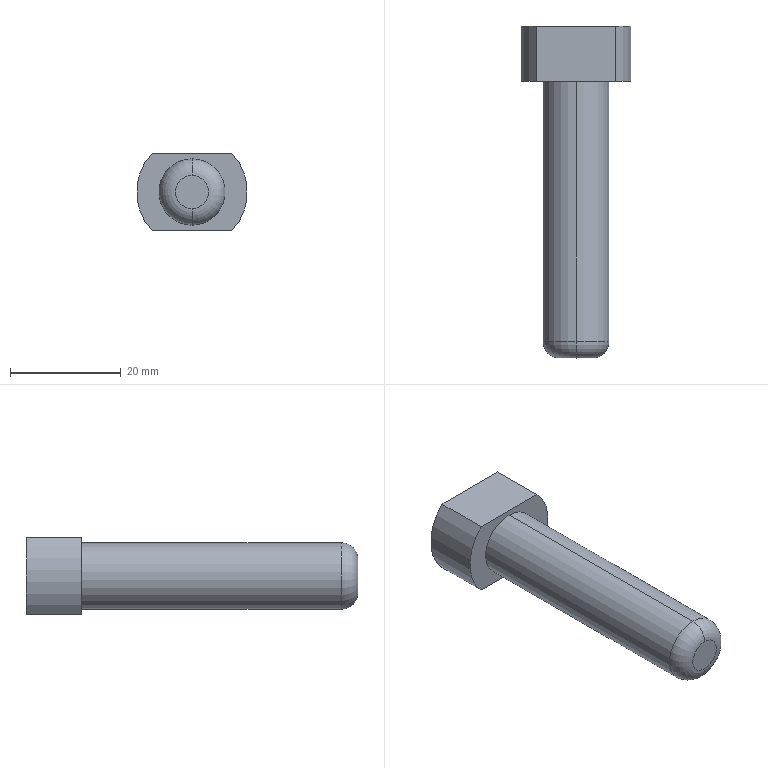Part | SolidWorks | features ICE 2, Extrusion 1, Fillet 1 | 1 solid | 11 faces | box 20 x 60 x 14 mm | volume 8141 mm3 | plane 5 | cylinder 4 | torus 2 | commonest cylinder face diameters 12 x2 20 x2
STEP:
#1=CARTESIAN_POINT('',(0.,-30.,-3.));
#2=VERTEX_POINT('',#1);
#3=CARTESIAN_POINT('',(0.,-30.,3.));
#4=VERTEX_POINT('',#3);
#5=CARTESIAN_POINT('',(0.,-30.,0.));
#6=DIRECTION('',(0.,-1.,0.));
#7=DIRECTION('',(0.,0.,1.));
#8=AXIS2_PLACEMENT_3D('',#5,#6,#7);
#9=CIRCLE('',#8,3.);
#10=EDGE_CURVE('',#2,#4,#9,.T.);
#11=ORIENTED_EDGE('',*,*,#10,.F.);
#12=CARTESIAN_POINT('',(0.,-27.,-6.));
#13=VERTEX_POINT('',#12);
#14=CARTESIAN_POINT('',(0.,-27.,-3.));
#15=DIRECTION('',(1.,0.,0.));
#16=DIRECTION('',(0.,0.,-1.));
#17=AXIS2_PLACEMENT_3D('',#14,#15,#16);
#18=CIRCLE('',#17,3.);
#19=EDGE_CURVE('',#2,#13,#18,.T.);
#20=ORIENTED_EDGE('',*,*,#19,.T.);
#21=CARTESIAN_POINT('',(0.,-27.,6.));
#22=VERTEX_POINT('',#21);
#23=CARTESIAN_POINT('',(0.,-27.,0.));
#24=DIRECTION('',(0.,1.,0.));
#25=DIRECTION('',(0.,0.,1.));
#26=AXIS2_PLACEMENT_3D('',#23,#24,#25);
#27=CIRCLE('',#26,6.);
#28=EDGE_CURVE('',#22,#13,#27,.T.);
#29=ORIENTED_EDGE('',*,*,#28,.F.);
#30=CARTESIAN_POINT('',(0.,-27.,3.));
#31=DIRECTION('',(-1.,0.,0.));
#32=DIRECTION('',(0.,0.,1.));
#33=AXIS2_PLACEMENT_3D('',#30,#31,#32);
#34=CIRCLE('',#33,3.);
#35=EDGE_CURVE('',#4,#22,#34,.T.);
#36=ORIENTED_EDGE('',*,*,#35,.F.);
#37=EDGE_LOOP('',(#11,#20,#29,#36));
#38=FACE_OUTER_BOUND('',#37,.T.);
#39=CARTESIAN_POINT('',(0.,-27.,0.));
#40=DIRECTION('',(0.,1.,0.));
#41=DIRECTION('',(0.,0.,1.));
#42=AXIS2_PLACEMENT_3D('',#39,#40,#41);
#43=TOROIDAL_SURFACE('',#42,3.,3.);
#44=ADVANCED_FACE('',(#38),#43,.T.);
#45=CARTESIAN_POINT('',(0.,20.,-6.));
#46=VERTEX_POINT('',#45);
#47=CARTESIAN_POINT('',(0.,20.,6.));
#48=VERTEX_POINT('',#47);
#49=CARTESIAN_POINT('',(0.,20.,0.));
#50=DIRECTION('',(0.,-1.,0.));
#51=DIRECTION('',(0.,0.,-1.));
#52=AXIS2_PLACEMENT_3D('',#49,#50,#51);
#53=CIRCLE('',#52,6.);
#54=EDGE_CURVE('',#46,#48,#53,.T.);
#55=ORIENTED_EDGE('',*,*,#54,.T.);
#56=CARTESIAN_POINT('',(0.,20.,6.));
#57=DIRECTION('',(0.,-1.,0.));
#58=VECTOR('',#57,1000.);
#59=LINE('',#56,#58);
#60=EDGE_CURVE('',#48,#22,#59,.T.);
#61=ORIENTED_EDGE('',*,*,#60,.T.);
#62=ORIENTED_EDGE('',*,*,#28,.T.);
#63=CARTESIAN_POINT('',(0.,20.,-6.));
#64=DIRECTION('',(0.,-1.,0.));
#65=VECTOR('',#64,1000.);
#66=LINE('',#63,#65);
#67=EDGE_CURVE('',#46,#13,#66,.T.);
#68=ORIENTED_EDGE('',*,*,#67,.F.);
#69=EDGE_LOOP('',(#55,#61,#62,#68));
#70=FACE_OUTER_BOUND('',#69,.T.);
#71=CARTESIAN_POINT('',(0.,20.,0.));
#72=DIRECTION('',(0.,-1.,0.));
#73=DIRECTION('',(0.,0.,-1.));
#74=AXIS2_PLACEMENT_3D('',#71,#72,#73);
#75=CYLINDRICAL_SURFACE('',#74,6.);
#76=ADVANCED_FACE('',(#70),#75,.T.);
#77=CARTESIAN_POINT('',(-7.141,30.,-7.));
#78=VERTEX_POINT('',#77);
#79=CARTESIAN_POINT('',(-7.141,30.,7.));
#80=VERTEX_POINT('',#79);
#81=CARTESIAN_POINT('',(0.,30.,0.));
#82=DIRECTION('',(0.,1.,0.));
#83=DIRECTION('',(0.,0.,1.));
#84=AXIS2_PLACEMENT_3D('',#81,#82,#83);
#85=CIRCLE('',#84,10.);
#86=EDGE_CURVE('',#78,#80,#85,.T.);
#87=ORIENTED_EDGE('',*,*,#86,.F.);
#88=CARTESIAN_POINT('',(-7.141,20.,-7.));
#89=VERTEX_POINT('',#88);
#90=CARTESIAN_POINT('',(-7.141,20.,-7.));
#91=DIRECTION('',(0.,1.,0.));
#92=VECTOR('',#91,1000.);
#93=LINE('',#90,#92);
#94=EDGE_CURVE('',#89,#78,#93,.T.);
#95=ORIENTED_EDGE('',*,*,#94,.F.);
#96=CARTESIAN_POINT('',(-7.141,20.,7.));
#97=VERTEX_POINT('',#96);
#98=CARTESIAN_POINT('',(0.,20.,0.));
#99=DIRECTION('',(0.,-1.,0.));
#100=DIRECTION('',(0.,0.,-1.));
#101=AXIS2_PLACEMENT_3D('',#98,#99,#100);
#102=CIRCLE('',#101,10.);
#103=EDGE_CURVE('',#97,#89,#102,.T.);
#104=ORIENTED_EDGE('',*,*,#103,.F.);
#105=CARTESIAN_POINT('',(-7.141,20.,7.));
#106=DIRECTION('',(0.,1.,0.));
#107=VECTOR('',#106,1000.);
#108=LINE('',#105,#107);
#109=EDGE_CURVE('',#97,#80,#108,.T.);
#110=ORIENTED_EDGE('',*,*,#109,.T.);
#111=EDGE_LOOP('',(#87,#95,#104,#110));
#112=FACE_OUTER_BOUND('',#111,.T.);
#113=CARTESIAN_POINT('',(0.,30.,0.));
#114=DIRECTION('',(0.,-1.,0.));
#115=DIRECTION('',(0.,0.,-1.));
#116=AXIS2_PLACEMENT_3D('',#113,#114,#115);
#117=CYLINDRICAL_SURFACE('',#116,10.);
#118=ADVANCED_FACE('',(#112),#117,.T.);
#119=CARTESIAN_POINT('',(7.141,20.,-7.));
#120=VERTEX_POINT('',#119);
#121=CARTESIAN_POINT('',(7.141,20.,7.));
#122=VERTEX_POINT('',#121);
#123=CARTESIAN_POINT('',(0.,20.,0.));
#124=DIRECTION('',(0.,-1.,0.));
#125=DIRECTION('',(0.,0.,-1.));
#126=AXIS2_PLACEMENT_3D('',#123,#124,#125);
#127=CIRCLE('',#126,10.);
#128=EDGE_CURVE('',#120,#122,#127,.T.);
#129=ORIENTED_EDGE('',*,*,#128,.F.);
#130=CARTESIAN_POINT('',(7.141,30.,-7.));
#131=VERTEX_POINT('',#130);
#132=CARTESIAN_POINT('',(7.141,20.,-7.));
#133=DIRECTION('',(0.,1.,0.));
#134=VECTOR('',#133,1000.);
#135=LINE('',#132,#134);
#136=EDGE_CURVE('',#120,#131,#135,.T.);
#137=ORIENTED_EDGE('',*,*,#136,.T.);
#138=CARTESIAN_POINT('',(7.141,30.,7.));
#139=VERTEX_POINT('',#138);
#140=CARTESIAN_POINT('',(0.,30.,0.));
#141=DIRECTION('',(0.,1.,0.));
#142=DIRECTION('',(0.,0.,1.));
#143=AXIS2_PLACEMENT_3D('',#140,#141,#142);
#144=CIRCLE('',#143,10.);
#145=EDGE_CURVE('',#139,#131,#144,.T.);
#146=ORIENTED_EDGE('',*,*,#145,.F.);
#147=CARTESIAN_POINT('',(7.141,20.,7.));
#148=DIRECTION('',(0.,1.,0.));
#149=VECTOR('',#148,1000.);
#150=LINE('',#147,#149);
#151=EDGE_CURVE('',#122,#139,#150,.T.);
#152=ORIENTED_EDGE('',*,*,#151,.F.);
#153=EDGE_LOOP('',(#129,#137,#146,#152));
#154=FACE_OUTER_BOUND('',#153,.T.);
#155=CARTESIAN_POINT('',(0.,30.,0.));
#156=DIRECTION('',(0.,-1.,0.));
#157=DIRECTION('',(0.,0.,-1.));
#158=AXIS2_PLACEMENT_3D('',#155,#156,#157);
#159=CYLINDRICAL_SURFACE('',#158,10.);
#160=ADVANCED_FACE('',(#154),#159,.T.);
#161=CARTESIAN_POINT('',(-7.141,30.,-7.));
#162=DIRECTION('',(1.,0.,0.));
#163=VECTOR('',#162,1000.);
#164=LINE('',#161,#163);
#165=EDGE_CURVE('',#78,#131,#164,.T.);
#166=ORIENTED_EDGE('',*,*,#165,.F.);
#167=ORIENTED_EDGE('',*,*,#86,.T.);
#168=CARTESIAN_POINT('',(-7.141,30.,7.));
#169=DIRECTION('',(-1.,0.,0.));
#170=VECTOR('',#169,1000.);
#171=LINE('',#168,#170);
#172=EDGE_CURVE('',#139,#80,#171,.T.);
#173=ORIENTED_EDGE('',*,*,#172,.F.);
#174=ORIENTED_EDGE('',*,*,#145,.T.);
#175=EDGE_LOOP('',(#166,#167,#173,#174));
#176=FACE_OUTER_BOUND('',#175,.T.);
#177=CARTESIAN_POINT('',(0.,30.,0.));
#178=DIRECTION('',(0.,1.,0.));
#179=DIRECTION('',(0.,0.,1.));
#180=AXIS2_PLACEMENT_3D('',#177,#178,#179);
#181=PLANE('',#180);
#182=ADVANCED_FACE('',(#176),#181,.T.);
#183=CARTESIAN_POINT('',(-7.141,20.,-7.));
#184=DIRECTION('',(1.,0.,0.));
#185=VECTOR('',#184,1000.);
#186=LINE('',#183,#185);
#187=EDGE_CURVE('',#89,#120,#186,.T.);
#188=ORIENTED_EDGE('',*,*,#187,.T.);
#189=ORIENTED_EDGE('',*,*,#128,.T.);
#190=CARTESIAN_POINT('',(-7.141,20.,7.));
#191=DIRECTION('',(-1.,0.,0.));
#192=VECTOR('',#191,1000.);
#193=LINE('',#190,#192);
#194=EDGE_CURVE('',#122,#97,#193,.T.);
#195=ORIENTED_EDGE('',*,*,#194,.T.);
#196=ORIENTED_EDGE('',*,*,#103,.T.);
#197=EDGE_LOOP('',(#188,#189,#195,#196));
#198=FACE_OUTER_BOUND('',#197,.T.);
#199=ORIENTED_EDGE('',*,*,#54,.F.);
#200=CARTESIAN_POINT('',(0.,20.,0.));
#201=DIRECTION('',(0.,-1.,0.));
#202=DIRECTION('',(0.,0.,-1.));
#203=AXIS2_PLACEMENT_3D('',#200,#201,#202);
#204=CIRCLE('',#203,6.);
#205=EDGE_CURVE('',#48,#46,#204,.T.);
#206=ORIENTED_EDGE('',*,*,#205,.F.);
#207=EDGE_LOOP('',(#199,#206));
#208=FACE_BOUND('',#207,.T.);
#209=CARTESIAN_POINT('',(0.,20.,0.));
#210=DIRECTION('',(0.,-1.,0.));
#211=DIRECTION('',(0.,0.,-1.));
#212=AXIS2_PLACEMENT_3D('',#209,#210,#211);
#213=PLANE('',#212);
#214=ADVANCED_FACE('',(#198,#208),#213,.T.);
#215=ORIENTED_EDGE('',*,*,#60,.F.);
#216=ORIENTED_EDGE('',*,*,#205,.T.);
#217=ORIENTED_EDGE('',*,*,#67,.T.);
#218=CARTESIAN_POINT('',(0.,-27.,0.));
#219=DIRECTION('',(0.,1.,0.));
#220=DIRECTION('',(0.,0.,1.));
#221=AXIS2_PLACEMENT_3D('',#218,#219,#220);
#222=CIRCLE('',#221,6.);
#223=EDGE_CURVE('',#13,#22,#222,.T.);
#224=ORIENTED_EDGE('',*,*,#223,.T.);
#225=EDGE_LOOP('',(#215,#216,#217,#224));
#226=FACE_OUTER_BOUND('',#225,.T.);
#227=CARTESIAN_POINT('',(0.,20.,0.));
#228=DIRECTION('',(0.,-1.,0.));
#229=DIRECTION('',(0.,0.,-1.));
#230=AXIS2_PLACEMENT_3D('',#227,#228,#229);
#231=CYLINDRICAL_SURFACE('',#230,6.);
#232=ADVANCED_FACE('',(#226),#231,.T.);
#233=CARTESIAN_POINT('',(0.,-30.,0.));
#234=DIRECTION('',(0.,-1.,0.));
#235=DIRECTION('',(0.,0.,1.));
#236=AXIS2_PLACEMENT_3D('',#233,#234,#235);
#237=CIRCLE('',#236,3.);
#238=EDGE_CURVE('',#4,#2,#237,.T.);
#239=ORIENTED_EDGE('',*,*,#238,.T.);
#240=ORIENTED_EDGE('',*,*,#10,.T.);
#241=EDGE_LOOP('',(#239,#240));
#242=FACE_OUTER_BOUND('',#241,.T.);
#243=CARTESIAN_POINT('',(0.,-30.,0.));
#244=DIRECTION('',(0.,1.,0.));
#245=DIRECTION('',(0.,0.,1.));
#246=AXIS2_PLACEMENT_3D('',#243,#244,#245);
#247=PLANE('',#246);
#248=ADVANCED_FACE('',(#242),#247,.F.);
#249=ORIENTED_EDGE('',*,*,#19,.F.);
#250=ORIENTED_EDGE('',*,*,#238,.F.);
#251=ORIENTED_EDGE('',*,*,#35,.T.);
#252=ORIENTED_EDGE('',*,*,#223,.F.);
#253=EDGE_LOOP('',(#249,#250,#251,#252));
#254=FACE_OUTER_BOUND('',#253,.T.);
#255=CARTESIAN_POINT('',(0.,-27.,0.));
#256=DIRECTION('',(0.,1.,0.));
#257=DIRECTION('',(0.,0.,1.));
#258=AXIS2_PLACEMENT_3D('',#255,#256,#257);
#259=TOROIDAL_SURFACE('',#258,3.,3.);
#260=ADVANCED_FACE('',(#254),#259,.T.);
#261=ORIENTED_EDGE('',*,*,#172,.T.);
#262=ORIENTED_EDGE('',*,*,#109,.F.);
#263=ORIENTED_EDGE('',*,*,#194,.F.);
#264=ORIENTED_EDGE('',*,*,#151,.T.);
#265=EDGE_LOOP('',(#261,#262,#263,#264));
#266=FACE_OUTER_BOUND('',#265,.T.);
#267=CARTESIAN_POINT('',(-7.141,20.,7.));
#268=DIRECTION('',(0.,0.,-1.));
#269=DIRECTION('',(-1.,0.,0.));
#270=AXIS2_PLACEMENT_3D('',#267,#268,#269);
#271=PLANE('',#270);
#272=ADVANCED_FACE('',(#266),#271,.F.);
#273=ORIENTED_EDGE('',*,*,#165,.T.);
#274=ORIENTED_EDGE('',*,*,#136,.F.);
#275=ORIENTED_EDGE('',*,*,#187,.F.);
#276=ORIENTED_EDGE('',*,*,#94,.T.);
#277=EDGE_LOOP('',(#273,#274,#275,#276));
#278=FACE_OUTER_BOUND('',#277,.T.);
#279=CARTESIAN_POINT('',(-7.141,20.,-7.));
#280=DIRECTION('',(0.,0.,1.));
#281=DIRECTION('',(1.,0.,0.));
#282=AXIS2_PLACEMENT_3D('',#279,#280,#281);
#283=PLANE('',#282);
#284=ADVANCED_FACE('',(#278),#283,.F.);
#285=CLOSED_SHELL('',(#44,#76,#118,#160,#182,#214,#232,#248,#260,#272,#284));
#286=MANIFOLD_SOLID_BREP('',#285);
#287=CARTESIAN_POINT('',(0.,0.,0.));
#288=DIRECTION('',(0.,0.,1.));
#289=DIRECTION('',(1.,0.,0.));
#290=AXIS2_PLACEMENT_3D('',#287,#288,#289);
#291=(LENGTH_UNIT()NAMED_UNIT(*)SI_UNIT(.MILLI.,.METRE.));
#292=UNCERTAINTY_MEASURE_WITH_UNIT(LENGTH_MEASURE(0.00001),#291,'','');
#293=(NAMED_UNIT(*)PLANE_ANGLE_UNIT()SI_UNIT($,.RADIAN.));
#294=(NAMED_UNIT(*)SI_UNIT($,.STERADIAN.)SOLID_ANGLE_UNIT());
#295=(GEOMETRIC_REPRESENTATION_CONTEXT(3)GLOBAL_UNCERTAINTY_ASSIGNED_CONTEXT((#292))GLOBAL_UNIT_ASSIGNED_CONTEXT((#291,#293,#294))REPRESENTATION_CONTEXT('',''));
#296=ADVANCED_BREP_SHAPE_REPRESENTATION('',(#286,#290),#295);